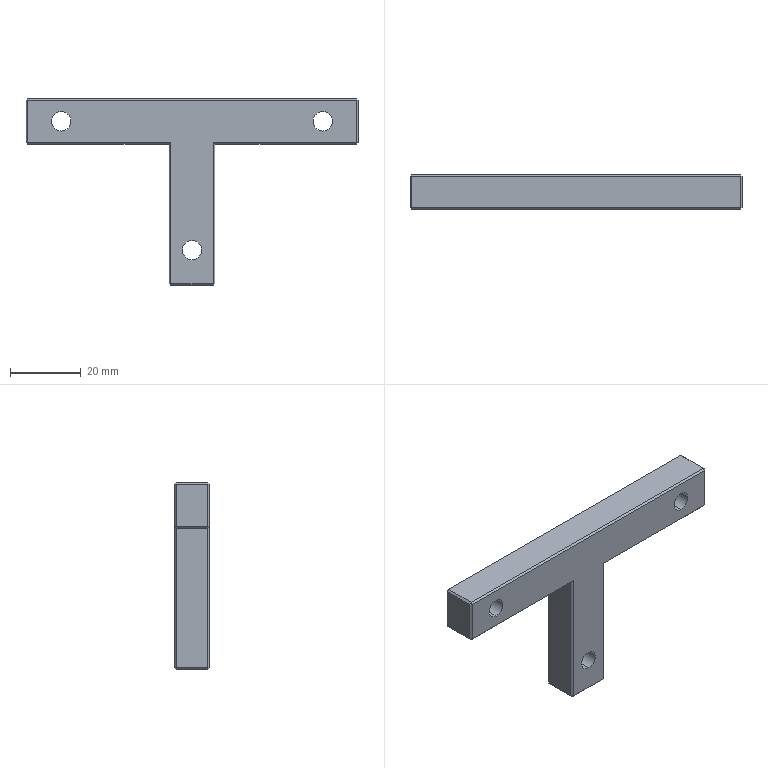Part | 1 solid | 59 faces | box 94 x 10 x 53 mm | volume 15677 mm3 | plane 47 | cylinder 12 | commonest cylinder face diameters 5.5 x6 10 x6
STEP:
#1=CARTESIAN_POINT('',(-37.,4.3,1.5));
#2=VERTEX_POINT('',#1);
#3=CARTESIAN_POINT('',(-37.,4.3,11.5));
#4=VERTEX_POINT('',#3);
#5=CARTESIAN_POINT('',(-37.,4.3,6.5));
#6=DIRECTION('',(0.,1.,0.));
#7=DIRECTION('',(0.,0.,1.));
#8=AXIS2_PLACEMENT_3D('',#5,#6,#7);
#9=CIRCLE('',#8,5.);
#10=EDGE_CURVE('',#2,#4,#9,.T.);
#11=ORIENTED_EDGE('',*,*,#10,.F.);
#12=CARTESIAN_POINT('',(-37.,10.,1.5));
#13=VERTEX_POINT('',#12);
#14=CARTESIAN_POINT('',(-37.,10.,1.5));
#15=DIRECTION('',(0.,1.,0.));
#16=VECTOR('',#15,1000.);
#17=LINE('',#14,#16);
#18=EDGE_CURVE('',#2,#13,#17,.T.);
#19=ORIENTED_EDGE('',*,*,#18,.T.);
#20=CARTESIAN_POINT('',(-37.,10.,11.5));
#21=VERTEX_POINT('',#20);
#22=CARTESIAN_POINT('',(-37.,10.,6.5));
#23=DIRECTION('',(0.,1.,0.));
#24=DIRECTION('',(0.,0.,1.));
#25=AXIS2_PLACEMENT_3D('',#22,#23,#24);
#26=CIRCLE('',#25,5.);
#27=EDGE_CURVE('',#13,#21,#26,.T.);
#28=ORIENTED_EDGE('',*,*,#27,.T.);
#29=CARTESIAN_POINT('',(-37.,10.,11.5));
#30=DIRECTION('',(0.,1.,0.));
#31=VECTOR('',#30,1000.);
#32=LINE('',#29,#31);
#33=EDGE_CURVE('',#4,#21,#32,.T.);
#34=ORIENTED_EDGE('',*,*,#33,.F.);
#35=EDGE_LOOP('',(#11,#19,#28,#34));
#36=FACE_OUTER_BOUND('',#35,.T.);
#37=CARTESIAN_POINT('',(-37.,10.,6.5));
#38=DIRECTION('',(0.,1.,0.));
#39=DIRECTION('',(0.,0.,1.));
#40=AXIS2_PLACEMENT_3D('',#37,#38,#39);
#41=CYLINDRICAL_SURFACE('',#40,5.);
#42=ADVANCED_FACE('',(#36),#41,.F.);
#43=CARTESIAN_POINT('',(-37.,0.,3.75));
#44=VERTEX_POINT('',#43);
#45=CARTESIAN_POINT('',(-37.,0.,9.25));
#46=VERTEX_POINT('',#45);
#47=CARTESIAN_POINT('',(-37.,0.,6.5));
#48=DIRECTION('',(0.,1.,0.));
#49=DIRECTION('',(0.,0.,1.));
#50=AXIS2_PLACEMENT_3D('',#47,#48,#49);
#51=CIRCLE('',#50,2.75);
#52=EDGE_CURVE('',#44,#46,#51,.T.);
#53=ORIENTED_EDGE('',*,*,#52,.F.);
#54=CARTESIAN_POINT('',(-37.,4.3,3.75));
#55=VERTEX_POINT('',#54);
#56=CARTESIAN_POINT('',(-37.,10.,3.75));
#57=DIRECTION('',(0.,1.,0.));
#58=VECTOR('',#57,1000.);
#59=LINE('',#56,#58);
#60=EDGE_CURVE('',#44,#55,#59,.T.);
#61=ORIENTED_EDGE('',*,*,#60,.T.);
#62=CARTESIAN_POINT('',(-37.,4.3,9.25));
#63=VERTEX_POINT('',#62);
#64=CARTESIAN_POINT('',(-37.,4.3,6.5));
#65=DIRECTION('',(0.,1.,0.));
#66=DIRECTION('',(0.,0.,1.));
#67=AXIS2_PLACEMENT_3D('',#64,#65,#66);
#68=CIRCLE('',#67,2.75);
#69=EDGE_CURVE('',#55,#63,#68,.T.);
#70=ORIENTED_EDGE('',*,*,#69,.T.);
#71=CARTESIAN_POINT('',(-37.,10.,9.25));
#72=DIRECTION('',(0.,1.,0.));
#73=VECTOR('',#72,1000.);
#74=LINE('',#71,#73);
#75=EDGE_CURVE('',#46,#63,#74,.T.);
#76=ORIENTED_EDGE('',*,*,#75,.F.);
#77=EDGE_LOOP('',(#53,#61,#70,#76));
#78=FACE_OUTER_BOUND('',#77,.T.);
#79=CARTESIAN_POINT('',(-37.,10.,6.5));
#80=DIRECTION('',(0.,1.,0.));
#81=DIRECTION('',(0.,0.,1.));
#82=AXIS2_PLACEMENT_3D('',#79,#80,#81);
#83=CYLINDRICAL_SURFACE('',#82,2.75);
#84=ADVANCED_FACE('',(#78),#83,.F.);
#85=CARTESIAN_POINT('',(37.,4.3,1.5));
#86=VERTEX_POINT('',#85);
#87=CARTESIAN_POINT('',(37.,4.3,11.5));
#88=VERTEX_POINT('',#87);
#89=CARTESIAN_POINT('',(37.,4.3,6.5));
#90=DIRECTION('',(0.,1.,0.));
#91=DIRECTION('',(0.,0.,1.));
#92=AXIS2_PLACEMENT_3D('',#89,#90,#91);
#93=CIRCLE('',#92,5.);
#94=EDGE_CURVE('',#86,#88,#93,.T.);
#95=ORIENTED_EDGE('',*,*,#94,.F.);
#96=CARTESIAN_POINT('',(37.,10.,1.5));
#97=VERTEX_POINT('',#96);
#98=CARTESIAN_POINT('',(37.,10.,1.5));
#99=DIRECTION('',(0.,1.,0.));
#100=VECTOR('',#99,1000.);
#101=LINE('',#98,#100);
#102=EDGE_CURVE('',#86,#97,#101,.T.);
#103=ORIENTED_EDGE('',*,*,#102,.T.);
#104=CARTESIAN_POINT('',(37.,10.,11.5));
#105=VERTEX_POINT('',#104);
#106=CARTESIAN_POINT('',(37.,10.,6.5));
#107=DIRECTION('',(0.,1.,0.));
#108=DIRECTION('',(0.,0.,1.));
#109=AXIS2_PLACEMENT_3D('',#106,#107,#108);
#110=CIRCLE('',#109,5.);
#111=EDGE_CURVE('',#97,#105,#110,.T.);
#112=ORIENTED_EDGE('',*,*,#111,.T.);
#113=CARTESIAN_POINT('',(37.,10.,11.5));
#114=DIRECTION('',(0.,1.,0.));
#115=VECTOR('',#114,1000.);
#116=LINE('',#113,#115);
#117=EDGE_CURVE('',#88,#105,#116,.T.);
#118=ORIENTED_EDGE('',*,*,#117,.F.);
#119=EDGE_LOOP('',(#95,#103,#112,#118));
#120=FACE_OUTER_BOUND('',#119,.T.);
#121=CARTESIAN_POINT('',(37.,10.,6.5));
#122=DIRECTION('',(0.,1.,0.));
#123=DIRECTION('',(0.,0.,1.));
#124=AXIS2_PLACEMENT_3D('',#121,#122,#123);
#125=CYLINDRICAL_SURFACE('',#124,5.);
#126=ADVANCED_FACE('',(#120),#125,.F.);
#127=CARTESIAN_POINT('',(37.,0.,3.75));
#128=VERTEX_POINT('',#127);
#129=CARTESIAN_POINT('',(37.,0.,9.25));
#130=VERTEX_POINT('',#129);
#131=CARTESIAN_POINT('',(37.,0.,6.5));
#132=DIRECTION('',(0.,1.,0.));
#133=DIRECTION('',(0.,0.,1.));
#134=AXIS2_PLACEMENT_3D('',#131,#132,#133);
#135=CIRCLE('',#134,2.75);
#136=EDGE_CURVE('',#128,#130,#135,.T.);
#137=ORIENTED_EDGE('',*,*,#136,.F.);
#138=CARTESIAN_POINT('',(37.,4.3,3.75));
#139=VERTEX_POINT('',#138);
#140=CARTESIAN_POINT('',(37.,10.,3.75));
#141=DIRECTION('',(0.,1.,0.));
#142=VECTOR('',#141,1000.);
#143=LINE('',#140,#142);
#144=EDGE_CURVE('',#128,#139,#143,.T.);
#145=ORIENTED_EDGE('',*,*,#144,.T.);
#146=CARTESIAN_POINT('',(37.,4.3,9.25));
#147=VERTEX_POINT('',#146);
#148=CARTESIAN_POINT('',(37.,4.3,6.5));
#149=DIRECTION('',(0.,1.,0.));
#150=DIRECTION('',(0.,0.,1.));
#151=AXIS2_PLACEMENT_3D('',#148,#149,#150);
#152=CIRCLE('',#151,2.75);
#153=EDGE_CURVE('',#139,#147,#152,.T.);
#154=ORIENTED_EDGE('',*,*,#153,.T.);
#155=CARTESIAN_POINT('',(37.,10.,9.25));
#156=DIRECTION('',(0.,1.,0.));
#157=VECTOR('',#156,1000.);
#158=LINE('',#155,#157);
#159=EDGE_CURVE('',#130,#147,#158,.T.);
#160=ORIENTED_EDGE('',*,*,#159,.F.);
#161=EDGE_LOOP('',(#137,#145,#154,#160));
#162=FACE_OUTER_BOUND('',#161,.T.);
#163=CARTESIAN_POINT('',(37.,10.,6.5));
#164=DIRECTION('',(0.,1.,0.));
#165=DIRECTION('',(0.,0.,1.));
#166=AXIS2_PLACEMENT_3D('',#163,#164,#165);
#167=CYLINDRICAL_SURFACE('',#166,2.75);
#168=ADVANCED_FACE('',(#162),#167,.F.);
#169=CARTESIAN_POINT('',(0.,4.3,-35.));
#170=VERTEX_POINT('',#169);
#171=CARTESIAN_POINT('',(0.,4.3,-25.));
#172=VERTEX_POINT('',#171);
#173=CARTESIAN_POINT('',(0.,4.3,-30.));
#174=DIRECTION('',(0.,1.,0.));
#175=DIRECTION('',(0.,0.,1.));
#176=AXIS2_PLACEMENT_3D('',#173,#174,#175);
#177=CIRCLE('',#176,5.);
#178=EDGE_CURVE('',#170,#172,#177,.T.);
#179=ORIENTED_EDGE('',*,*,#178,.F.);
#180=CARTESIAN_POINT('',(0.,10.,-35.));
#181=VERTEX_POINT('',#180);
#182=CARTESIAN_POINT('',(0.,10.,-35.));
#183=DIRECTION('',(0.,1.,0.));
#184=VECTOR('',#183,1000.);
#185=LINE('',#182,#184);
#186=EDGE_CURVE('',#170,#181,#185,.T.);
#187=ORIENTED_EDGE('',*,*,#186,.T.);
#188=CARTESIAN_POINT('',(0.,10.,-25.));
#189=VERTEX_POINT('',#188);
#190=CARTESIAN_POINT('',(0.,10.,-30.));
#191=DIRECTION('',(0.,1.,0.));
#192=DIRECTION('',(0.,0.,1.));
#193=AXIS2_PLACEMENT_3D('',#190,#191,#192);
#194=CIRCLE('',#193,5.);
#195=EDGE_CURVE('',#181,#189,#194,.T.);
#196=ORIENTED_EDGE('',*,*,#195,.T.);
#197=CARTESIAN_POINT('',(0.,10.,-25.));
#198=DIRECTION('',(0.,1.,0.));
#199=VECTOR('',#198,1000.);
#200=LINE('',#197,#199);
#201=EDGE_CURVE('',#172,#189,#200,.T.);
#202=ORIENTED_EDGE('',*,*,#201,.F.);
#203=EDGE_LOOP('',(#179,#187,#196,#202));
#204=FACE_OUTER_BOUND('',#203,.T.);
#205=CARTESIAN_POINT('',(0.,10.,-30.));
#206=DIRECTION('',(0.,1.,0.));
#207=DIRECTION('',(0.,0.,1.));
#208=AXIS2_PLACEMENT_3D('',#205,#206,#207);
#209=CYLINDRICAL_SURFACE('',#208,5.);
#210=ADVANCED_FACE('',(#204),#209,.F.);
#211=CARTESIAN_POINT('',(0.,0.,-32.75));
#212=VERTEX_POINT('',#211);
#213=CARTESIAN_POINT('',(0.,0.,-27.25));
#214=VERTEX_POINT('',#213);
#215=CARTESIAN_POINT('',(0.,0.,-30.));
#216=DIRECTION('',(0.,1.,0.));
#217=DIRECTION('',(0.,0.,1.));
#218=AXIS2_PLACEMENT_3D('',#215,#216,#217);
#219=CIRCLE('',#218,2.75);
#220=EDGE_CURVE('',#212,#214,#219,.T.);
#221=ORIENTED_EDGE('',*,*,#220,.F.);
#222=CARTESIAN_POINT('',(0.,4.3,-32.75));
#223=VERTEX_POINT('',#222);
#224=CARTESIAN_POINT('',(0.,10.,-32.75));
#225=DIRECTION('',(0.,1.,0.));
#226=VECTOR('',#225,1000.);
#227=LINE('',#224,#226);
#228=EDGE_CURVE('',#212,#223,#227,.T.);
#229=ORIENTED_EDGE('',*,*,#228,.T.);
#230=CARTESIAN_POINT('',(0.,4.3,-27.25));
#231=VERTEX_POINT('',#230);
#232=CARTESIAN_POINT('',(0.,4.3,-30.));
#233=DIRECTION('',(0.,1.,0.));
#234=DIRECTION('',(0.,0.,1.));
#235=AXIS2_PLACEMENT_3D('',#232,#233,#234);
#236=CIRCLE('',#235,2.75);
#237=EDGE_CURVE('',#223,#231,#236,.T.);
#238=ORIENTED_EDGE('',*,*,#237,.T.);
#239=CARTESIAN_POINT('',(0.,10.,-27.25));
#240=DIRECTION('',(0.,1.,0.));
#241=VECTOR('',#240,1000.);
#242=LINE('',#239,#241);
#243=EDGE_CURVE('',#214,#231,#242,.T.);
#244=ORIENTED_EDGE('',*,*,#243,.F.);
#245=EDGE_LOOP('',(#221,#229,#238,#244));
#246=FACE_OUTER_BOUND('',#245,.T.);
#247=CARTESIAN_POINT('',(0.,10.,-30.));
#248=DIRECTION('',(0.,1.,0.));
#249=DIRECTION('',(0.,0.,1.));
#250=AXIS2_PLACEMENT_3D('',#247,#248,#249);
#251=CYLINDRICAL_SURFACE('',#250,2.75);
#252=ADVANCED_FACE('',(#246),#251,.F.);
#253=CARTESIAN_POINT('',(-47.,0.54,0.54));
#254=VERTEX_POINT('',#253);
#255=CARTESIAN_POINT('',(-47.,0.54,12.46));
#256=VERTEX_POINT('',#255);
#257=CARTESIAN_POINT('',(-47.,0.54,13.));
#258=DIRECTION('',(0.,0.,1.));
#259=VECTOR('',#258,1000.);
#260=LINE('',#257,#259);
#261=EDGE_CURVE('',#254,#256,#260,.T.);
#262=ORIENTED_EDGE('',*,*,#261,.T.);
#263=CARTESIAN_POINT('',(-47.,9.46,12.46));
#264=VERTEX_POINT('',#263);
#265=CARTESIAN_POINT('',(-47.,10.,12.46));
#266=DIRECTION('',(0.,1.,0.));
#267=VECTOR('',#266,1000.);
#268=LINE('',#265,#267);
#269=EDGE_CURVE('',#256,#264,#268,.T.);
#270=ORIENTED_EDGE('',*,*,#269,.T.);
#271=CARTESIAN_POINT('',(-47.,9.46,0.54));
#272=VERTEX_POINT('',#271);
#273=CARTESIAN_POINT('',(-47.,9.46,13.));
#274=DIRECTION('',(0.,0.,-1.));
#275=VECTOR('',#274,1000.);
#276=LINE('',#273,#275);
#277=EDGE_CURVE('',#264,#272,#276,.T.);
#278=ORIENTED_EDGE('',*,*,#277,.T.);
#279=CARTESIAN_POINT('',(-47.,10.,0.54));
#280=DIRECTION('',(0.,-1.,0.));
#281=VECTOR('',#280,1000.);
#282=LINE('',#279,#281);
#283=EDGE_CURVE('',#272,#254,#282,.T.);
#284=ORIENTED_EDGE('',*,*,#283,.T.);
#285=EDGE_LOOP('',(#262,#270,#278,#284));
#286=FACE_OUTER_BOUND('',#285,.T.);
#287=CARTESIAN_POINT('',(-47.,10.,13.));
#288=DIRECTION('',(1.,0.,0.));
#289=DIRECTION('',(0.,0.,-1.));
#290=AXIS2_PLACEMENT_3D('',#287,#288,#289);
#291=PLANE('',#290);
#292=ADVANCED_FACE('',(#286),#291,.F.);
#293=CARTESIAN_POINT('',(46.46,9.46,13.));
#294=VERTEX_POINT('',#293);
#295=CARTESIAN_POINT('',(-46.46,9.46,13.));
#296=VERTEX_POINT('',#295);
#297=CARTESIAN_POINT('',(47.,9.46,13.));
#298=DIRECTION('',(-1.,0.,0.));
#299=VECTOR('',#298,1000.);
#300=LINE('',#297,#299);
#301=EDGE_CURVE('',#294,#296,#300,.T.);
#302=ORIENTED_EDGE('',*,*,#301,.T.);
#303=CARTESIAN_POINT('',(-46.46,0.54,13.));
#304=VERTEX_POINT('',#303);
#305=CARTESIAN_POINT('',(-46.46,10.,13.));
#306=DIRECTION('',(0.,-1.,0.));
#307=VECTOR('',#306,1000.);
#308=LINE('',#305,#307);
#309=EDGE_CURVE('',#296,#304,#308,.T.);
#310=ORIENTED_EDGE('',*,*,#309,.T.);
#311=CARTESIAN_POINT('',(46.46,0.54,13.));
#312=VERTEX_POINT('',#311);
#313=CARTESIAN_POINT('',(47.,0.54,13.));
#314=DIRECTION('',(1.,0.,0.));
#315=VECTOR('',#314,1000.);
#316=LINE('',#313,#315);
#317=EDGE_CURVE('',#304,#312,#316,.T.);
#318=ORIENTED_EDGE('',*,*,#317,.T.);
#319=CARTESIAN_POINT('',(46.46,10.,13.));
#320=DIRECTION('',(0.,1.,0.));
#321=VECTOR('',#320,1000.);
#322=LINE('',#319,#321);
#323=EDGE_CURVE('',#312,#294,#322,.T.);
#324=ORIENTED_EDGE('',*,*,#323,.T.);
#325=EDGE_LOOP('',(#302,#310,#318,#324));
#326=FACE_OUTER_BOUND('',#325,.T.);
#327=CARTESIAN_POINT('',(47.,10.,13.));
#328=DIRECTION('',(0.,0.,-1.));
#329=DIRECTION('',(-1.,0.,0.));
#330=AXIS2_PLACEMENT_3D('',#327,#328,#329);
#331=PLANE('',#330);
#332=ADVANCED_FACE('',(#326),#331,.F.);
#333=CARTESIAN_POINT('',(47.,9.46,0.54));
#334=VERTEX_POINT('',#333);
#335=CARTESIAN_POINT('',(47.,9.46,12.46));
#336=VERTEX_POINT('',#335);
#337=CARTESIAN_POINT('',(47.,9.46,0.));
#338=DIRECTION('',(0.,0.,1.));
#339=VECTOR('',#338,1000.);
#340=LINE('',#337,#339);
#341=EDGE_CURVE('',#334,#336,#340,.T.);
#342=ORIENTED_EDGE('',*,*,#341,.T.);
#343=CARTESIAN_POINT('',(47.,0.54,12.46));
#344=VERTEX_POINT('',#343);
#345=CARTESIAN_POINT('',(47.,10.,12.46));
#346=DIRECTION('',(0.,-1.,0.));
#347=VECTOR('',#346,1000.);
#348=LINE('',#345,#347);
#349=EDGE_CURVE('',#336,#344,#348,.T.);
#350=ORIENTED_EDGE('',*,*,#349,.T.);
#351=CARTESIAN_POINT('',(47.,0.54,0.54));
#352=VERTEX_POINT('',#351);
#353=CARTESIAN_POINT('',(47.,0.54,0.));
#354=DIRECTION('',(0.,0.,-1.));
#355=VECTOR('',#354,1000.);
#356=LINE('',#353,#355);
#357=EDGE_CURVE('',#344,#352,#356,.T.);
#358=ORIENTED_EDGE('',*,*,#357,.T.);
#359=CARTESIAN_POINT('',(47.,10.,0.54));
#360=DIRECTION('',(0.,1.,0.));
#361=VECTOR('',#360,1000.);
#362=LINE('',#359,#361);
#363=EDGE_CURVE('',#352,#334,#362,.T.);
#364=ORIENTED_EDGE('',*,*,#363,.T.);
#365=EDGE_LOOP('',(#342,#350,#358,#364));
#366=FACE_OUTER_BOUND('',#365,.T.);
#367=CARTESIAN_POINT('',(47.,10.,0.));
#368=DIRECTION('',(-1.,0.,0.));
#369=DIRECTION('',(0.,0.,1.));
#370=AXIS2_PLACEMENT_3D('',#367,#368,#369);
#371=PLANE('',#370);
#372=ADVANCED_FACE('',(#366),#371,.F.);
#373=CARTESIAN_POINT('',(46.46,9.46,0.));
#374=VERTEX_POINT('',#373);
#375=CARTESIAN_POINT('',(46.46,0.54,0.));
#376=VERTEX_POINT('',#375);
#377=CARTESIAN_POINT('',(46.46,10.,0.));
#378=DIRECTION('',(0.,-1.,0.));
#379=VECTOR('',#378,1000.);
#380=LINE('',#377,#379);
#381=EDGE_CURVE('',#374,#376,#380,.T.);
#382=ORIENTED_EDGE('',*,*,#381,.T.);
#383=CARTESIAN_POINT('',(6.5,0.54,0.));
#384=VERTEX_POINT('',#383);
#385=CARTESIAN_POINT('',(6.5,0.54,0.));
#386=DIRECTION('',(-1.,0.,0.));
#387=VECTOR('',#386,1000.);
#388=LINE('',#385,#387);
#389=EDGE_CURVE('',#376,#384,#388,.T.);
#390=ORIENTED_EDGE('',*,*,#389,.T.);
#391=CARTESIAN_POINT('',(6.5,9.46,0.));
#392=VERTEX_POINT('',#391);
#393=CARTESIAN_POINT('',(6.5,10.,0.));
#394=DIRECTION('',(0.,-1.,0.));
#395=VECTOR('',#394,1000.);
#396=LINE('',#393,#395);
#397=EDGE_CURVE('',#392,#384,#396,.T.);
#398=ORIENTED_EDGE('',*,*,#397,.F.);
#399=CARTESIAN_POINT('',(6.5,9.46,0.));
#400=DIRECTION('',(1.,0.,0.));
#401=VECTOR('',#400,1000.);
#402=LINE('',#399,#401);
#403=EDGE_CURVE('',#392,#374,#402,.T.);
#404=ORIENTED_EDGE('',*,*,#403,.T.);
#405=EDGE_LOOP('',(#382,#390,#398,#404));
#406=FACE_OUTER_BOUND('',#405,.T.);
#407=CARTESIAN_POINT('',(6.5,10.,0.));
#408=DIRECTION('',(0.,0.,1.));
#409=DIRECTION('',(1.,0.,0.));
#410=AXIS2_PLACEMENT_3D('',#407,#408,#409);
#411=PLANE('',#410);
#412=ADVANCED_FACE('',(#406),#411,.F.);
#413=ORIENTED_EDGE('',*,*,#397,.T.);
#414=CARTESIAN_POINT('',(6.5,0.54,-39.46));
#415=VERTEX_POINT('',#414);
#416=CARTESIAN_POINT('',(6.5,0.54,-40.));
#417=DIRECTION('',(0.,0.,-1.));
#418=VECTOR('',#417,1000.);
#419=LINE('',#416,#418);
#420=EDGE_CURVE('',#384,#415,#419,.T.);
#421=ORIENTED_EDGE('',*,*,#420,.T.);
#422=CARTESIAN_POINT('',(6.5,9.46,-39.46));
#423=VERTEX_POINT('',#422);
#424=CARTESIAN_POINT('',(6.5,10.,-39.46));
#425=DIRECTION('',(0.,1.,0.));
#426=VECTOR('',#425,1000.);
#427=LINE('',#424,#426);
#428=EDGE_CURVE('',#415,#423,#427,.T.);
#429=ORIENTED_EDGE('',*,*,#428,.T.);
#430=CARTESIAN_POINT('',(6.5,9.46,-40.));
#431=DIRECTION('',(0.,0.,1.));
#432=VECTOR('',#431,1000.);
#433=LINE('',#430,#432);
#434=EDGE_CURVE('',#423,#392,#433,.T.);
#435=ORIENTED_EDGE('',*,*,#434,.T.);
#436=EDGE_LOOP('',(#413,#421,#429,#435));
#437=FACE_OUTER_BOUND('',#436,.T.);
#438=CARTESIAN_POINT('',(6.5,10.,-40.));
#439=DIRECTION('',(-1.,0.,0.));
#440=DIRECTION('',(0.,0.,1.));
#441=AXIS2_PLACEMENT_3D('',#438,#439,#440);
#442=PLANE('',#441);
#443=ADVANCED_FACE('',(#437),#442,.F.);
#444=CARTESIAN_POINT('',(5.96,9.46,-40.));
#445=VERTEX_POINT('',#444);
#446=CARTESIAN_POINT('',(5.96,0.54,-40.));
#447=VERTEX_POINT('',#446);
#448=CARTESIAN_POINT('',(5.96,10.,-40.));
#449=DIRECTION('',(0.,-1.,0.));
#450=VECTOR('',#449,1000.);
#451=LINE('',#448,#450);
#452=EDGE_CURVE('',#445,#447,#451,.T.);
#453=ORIENTED_EDGE('',*,*,#452,.T.);
#454=CARTESIAN_POINT('',(-5.96,0.54,-40.));
#455=VERTEX_POINT('',#454);
#456=CARTESIAN_POINT('',(-6.5,0.54,-40.));
#457=DIRECTION('',(-1.,0.,0.));
#458=VECTOR('',#457,1000.);
#459=LINE('',#456,#458);
#460=EDGE_CURVE('',#447,#455,#459,.T.);
#461=ORIENTED_EDGE('',*,*,#460,.T.);
#462=CARTESIAN_POINT('',(-5.96,9.46,-40.));
#463=VERTEX_POINT('',#462);
#464=CARTESIAN_POINT('',(-5.96,10.,-40.));
#465=DIRECTION('',(0.,1.,0.));
#466=VECTOR('',#465,1000.);
#467=LINE('',#464,#466);
#468=EDGE_CURVE('',#455,#463,#467,.T.);
#469=ORIENTED_EDGE('',*,*,#468,.T.);
#470=CARTESIAN_POINT('',(-6.5,9.46,-40.));
#471=DIRECTION('',(1.,0.,0.));
#472=VECTOR('',#471,1000.);
#473=LINE('',#470,#472);
#474=EDGE_CURVE('',#463,#445,#473,.T.);
#475=ORIENTED_EDGE('',*,*,#474,.T.);
#476=EDGE_LOOP('',(#453,#461,#469,#475));
#477=FACE_OUTER_BOUND('',#476,.T.);
#478=CARTESIAN_POINT('',(-6.5,10.,-40.));
#479=DIRECTION('',(0.,0.,1.));
#480=DIRECTION('',(1.,0.,0.));
#481=AXIS2_PLACEMENT_3D('',#478,#479,#480);
#482=PLANE('',#481);
#483=ADVANCED_FACE('',(#477),#482,.F.);
#484=CARTESIAN_POINT('',(-6.5,9.46,-39.46));
#485=VERTEX_POINT('',#484);
#486=CARTESIAN_POINT('',(-6.5,0.54,-39.46));
#487=VERTEX_POINT('',#486);
#488=CARTESIAN_POINT('',(-6.5,10.,-39.46));
#489=DIRECTION('',(0.,-1.,0.));
#490=VECTOR('',#489,1000.);
#491=LINE('',#488,#490);
#492=EDGE_CURVE('',#485,#487,#491,.T.);
#493=ORIENTED_EDGE('',*,*,#492,.T.);
#494=CARTESIAN_POINT('',(-6.5,0.54,0.));
#495=VERTEX_POINT('',#494);
#496=CARTESIAN_POINT('',(-6.5,0.54,0.));
#497=DIRECTION('',(0.,0.,1.));
#498=VECTOR('',#497,1000.);
#499=LINE('',#496,#498);
#500=EDGE_CURVE('',#487,#495,#499,.T.);
#501=ORIENTED_EDGE('',*,*,#500,.T.);
#502=CARTESIAN_POINT('',(-6.5,9.46,0.));
#503=VERTEX_POINT('',#502);
#504=CARTESIAN_POINT('',(-6.5,10.,0.));
#505=DIRECTION('',(0.,-1.,0.));
#506=VECTOR('',#505,1000.);
#507=LINE('',#504,#506);
#508=EDGE_CURVE('',#503,#495,#507,.T.);
#509=ORIENTED_EDGE('',*,*,#508,.F.);
#510=CARTESIAN_POINT('',(-6.5,9.46,0.));
#511=DIRECTION('',(0.,0.,-1.));
#512=VECTOR('',#511,1000.);
#513=LINE('',#510,#512);
#514=EDGE_CURVE('',#503,#485,#513,.T.);
#515=ORIENTED_EDGE('',*,*,#514,.T.);
#516=EDGE_LOOP('',(#493,#501,#509,#515));
#517=FACE_OUTER_BOUND('',#516,.T.);
#518=CARTESIAN_POINT('',(-6.5,10.,0.));
#519=DIRECTION('',(1.,0.,0.));
#520=DIRECTION('',(0.,0.,-1.));
#521=AXIS2_PLACEMENT_3D('',#518,#519,#520);
#522=PLANE('',#521);
#523=ADVANCED_FACE('',(#517),#522,.F.);
#524=ORIENTED_EDGE('',*,*,#508,.T.);
#525=CARTESIAN_POINT('',(-46.46,0.54,0.));
#526=VERTEX_POINT('',#525);
#527=CARTESIAN_POINT('',(-47.,0.54,0.));
#528=DIRECTION('',(-1.,0.,0.));
#529=VECTOR('',#528,1000.);
#530=LINE('',#527,#529);
#531=EDGE_CURVE('',#495,#526,#530,.T.);
#532=ORIENTED_EDGE('',*,*,#531,.T.);
#533=CARTESIAN_POINT('',(-46.46,9.46,0.));
#534=VERTEX_POINT('',#533);
#535=CARTESIAN_POINT('',(-46.46,10.,0.));
#536=DIRECTION('',(0.,1.,0.));
#537=VECTOR('',#536,1000.);
#538=LINE('',#535,#537);
#539=EDGE_CURVE('',#526,#534,#538,.T.);
#540=ORIENTED_EDGE('',*,*,#539,.T.);
#541=CARTESIAN_POINT('',(-47.,9.46,0.));
#542=DIRECTION('',(1.,0.,0.));
#543=VECTOR('',#542,1000.);
#544=LINE('',#541,#543);
#545=EDGE_CURVE('',#534,#503,#544,.T.);
#546=ORIENTED_EDGE('',*,*,#545,.T.);
#547=EDGE_LOOP('',(#524,#532,#540,#546));
#548=FACE_OUTER_BOUND('',#547,.T.);
#549=CARTESIAN_POINT('',(-47.,10.,0.));
#550=DIRECTION('',(0.,0.,1.));
#551=DIRECTION('',(1.,0.,0.));
#552=AXIS2_PLACEMENT_3D('',#549,#550,#551);
#553=PLANE('',#552);
#554=ADVANCED_FACE('',(#548),#553,.F.);
#555=CARTESIAN_POINT('',(-37.,10.,6.5));
#556=DIRECTION('',(0.,1.,0.));
#557=DIRECTION('',(0.,0.,1.));
#558=AXIS2_PLACEMENT_3D('',#555,#556,#557);
#559=CIRCLE('',#558,5.);
#560=EDGE_CURVE('',#21,#13,#559,.T.);
#561=ORIENTED_EDGE('',*,*,#560,.F.);
#562=ORIENTED_EDGE('',*,*,#27,.F.);
#563=EDGE_LOOP('',(#561,#562));
#564=FACE_BOUND('',#563,.T.);
#565=CARTESIAN_POINT('',(37.,10.,6.5));
#566=DIRECTION('',(0.,1.,0.));
#567=DIRECTION('',(0.,0.,1.));
#568=AXIS2_PLACEMENT_3D('',#565,#566,#567);
#569=CIRCLE('',#568,5.);
#570=EDGE_CURVE('',#105,#97,#569,.T.);
#571=ORIENTED_EDGE('',*,*,#570,.F.);
#572=ORIENTED_EDGE('',*,*,#111,.F.);
#573=EDGE_LOOP('',(#571,#572));
#574=FACE_BOUND('',#573,.T.);
#575=CARTESIAN_POINT('',(0.,10.,-30.));
#576=DIRECTION('',(0.,1.,0.));
#577=DIRECTION('',(0.,0.,1.));
#578=AXIS2_PLACEMENT_3D('',#575,#576,#577);
#579=CIRCLE('',#578,5.);
#580=EDGE_CURVE('',#189,#181,#579,.T.);
#581=ORIENTED_EDGE('',*,*,#580,.F.);
#582=ORIENTED_EDGE('',*,*,#195,.F.);
#583=EDGE_LOOP('',(#581,#582));
#584=FACE_BOUND('',#583,.T.);
#585=CARTESIAN_POINT('',(-46.46,10.,0.54));
#586=VERTEX_POINT('',#585);
#587=CARTESIAN_POINT('',(-46.46,10.,12.46));
#588=VERTEX_POINT('',#587);
#589=CARTESIAN_POINT('',(-46.46,10.,0.));
#590=DIRECTION('',(0.,0.,1.));
#591=VECTOR('',#590,1000.);
#592=LINE('',#589,#591);
#593=EDGE_CURVE('',#586,#588,#592,.T.);
#594=ORIENTED_EDGE('',*,*,#593,.T.);
#595=CARTESIAN_POINT('',(46.46,10.,12.46));
#596=VERTEX_POINT('',#595);
#597=CARTESIAN_POINT('',(0.,10.,12.46));
#598=DIRECTION('',(1.,0.,0.));
#599=VECTOR('',#598,1000.);
#600=LINE('',#597,#599);
#601=EDGE_CURVE('',#588,#596,#600,.T.);
#602=ORIENTED_EDGE('',*,*,#601,.T.);
#603=CARTESIAN_POINT('',(46.46,10.,0.54));
#604=VERTEX_POINT('',#603);
#605=CARTESIAN_POINT('',(46.46,10.,0.));
#606=DIRECTION('',(0.,0.,-1.));
#607=VECTOR('',#606,1000.);
#608=LINE('',#605,#607);
#609=EDGE_CURVE('',#596,#604,#608,.T.);
#610=ORIENTED_EDGE('',*,*,#609,.T.);
#611=CARTESIAN_POINT('',(5.96,10.,0.54));
#612=VERTEX_POINT('',#611);
#613=CARTESIAN_POINT('',(0.,10.,0.54));
#614=DIRECTION('',(-1.,0.,0.));
#615=VECTOR('',#614,1000.);
#616=LINE('',#613,#615);
#617=EDGE_CURVE('',#604,#612,#616,.T.);
#618=ORIENTED_EDGE('',*,*,#617,.T.);
#619=CARTESIAN_POINT('',(5.96,10.,-39.46));
#620=VERTEX_POINT('',#619);
#621=CARTESIAN_POINT('',(5.96,10.,0.));
#622=DIRECTION('',(0.,0.,-1.));
#623=VECTOR('',#622,1000.);
#624=LINE('',#621,#623);
#625=EDGE_CURVE('',#612,#620,#624,.T.);
#626=ORIENTED_EDGE('',*,*,#625,.T.);
#627=CARTESIAN_POINT('',(-5.96,10.,-39.46));
#628=VERTEX_POINT('',#627);
#629=CARTESIAN_POINT('',(0.,10.,-39.46));
#630=DIRECTION('',(-1.,0.,0.));
#631=VECTOR('',#630,1000.);
#632=LINE('',#629,#631);
#633=EDGE_CURVE('',#620,#628,#632,.T.);
#634=ORIENTED_EDGE('',*,*,#633,.T.);
#635=CARTESIAN_POINT('',(-5.96,10.,0.54));
#636=VERTEX_POINT('',#635);
#637=CARTESIAN_POINT('',(-5.96,10.,0.));
#638=DIRECTION('',(0.,0.,1.));
#639=VECTOR('',#638,1000.);
#640=LINE('',#637,#639);
#641=EDGE_CURVE('',#628,#636,#640,.T.);
#642=ORIENTED_EDGE('',*,*,#641,.T.);
#643=CARTESIAN_POINT('',(0.,10.,0.54));
#644=DIRECTION('',(-1.,0.,0.));
#645=VECTOR('',#644,1000.);
#646=LINE('',#643,#645);
#647=EDGE_CURVE('',#636,#586,#646,.T.);
#648=ORIENTED_EDGE('',*,*,#647,.T.);
#649=EDGE_LOOP('',(#594,#602,#610,#618,#626,#634,#642,#648));
#650=FACE_OUTER_BOUND('',#649,.T.);
#651=CARTESIAN_POINT('',(0.,10.,0.));
#652=DIRECTION('',(0.,-1.,0.));
#653=DIRECTION('',(0.,0.,-1.));
#654=AXIS2_PLACEMENT_3D('',#651,#652,#653);
#655=PLANE('',#654);
#656=ADVANCED_FACE('',(#564,#574,#584,#650),#655,.F.);
#657=CARTESIAN_POINT('',(-37.,0.,6.5));
#658=DIRECTION('',(0.,1.,0.));
#659=DIRECTION('',(0.,0.,1.));
#660=AXIS2_PLACEMENT_3D('',#657,#658,#659);
#661=CIRCLE('',#660,2.75);
#662=EDGE_CURVE('',#46,#44,#661,.T.);
#663=ORIENTED_EDGE('',*,*,#662,.T.);
#664=ORIENTED_EDGE('',*,*,#52,.T.);
#665=EDGE_LOOP('',(#663,#664));
#666=FACE_BOUND('',#665,.T.);
#667=CARTESIAN_POINT('',(37.,0.,6.5));
#668=DIRECTION('',(0.,1.,0.));
#669=DIRECTION('',(0.,0.,1.));
#670=AXIS2_PLACEMENT_3D('',#667,#668,#669);
#671=CIRCLE('',#670,2.75);
#672=EDGE_CURVE('',#130,#128,#671,.T.);
#673=ORIENTED_EDGE('',*,*,#672,.T.);
#674=ORIENTED_EDGE('',*,*,#136,.T.);
#675=EDGE_LOOP('',(#673,#674));
#676=FACE_BOUND('',#675,.T.);
#677=CARTESIAN_POINT('',(0.,0.,-30.));
#678=DIRECTION('',(0.,1.,0.));
#679=DIRECTION('',(0.,0.,1.));
#680=AXIS2_PLACEMENT_3D('',#677,#678,#679);
#681=CIRCLE('',#680,2.75);
#682=EDGE_CURVE('',#214,#212,#681,.T.);
#683=ORIENTED_EDGE('',*,*,#682,.T.);
#684=ORIENTED_EDGE('',*,*,#220,.T.);
#685=EDGE_LOOP('',(#683,#684));
#686=FACE_BOUND('',#685,.T.);
#687=CARTESIAN_POINT('',(5.96,0.,-39.46));
#688=VERTEX_POINT('',#687);
#689=CARTESIAN_POINT('',(5.96,0.,0.54));
#690=VERTEX_POINT('',#689);
#691=CARTESIAN_POINT('',(5.96,0.,0.));
#692=DIRECTION('',(0.,0.,1.));
#693=VECTOR('',#692,1000.);
#694=LINE('',#691,#693);
#695=EDGE_CURVE('',#688,#690,#694,.T.);
#696=ORIENTED_EDGE('',*,*,#695,.T.);
#697=CARTESIAN_POINT('',(46.46,0.,0.54));
#698=VERTEX_POINT('',#697);
#699=CARTESIAN_POINT('',(47.,0.,0.54));
#700=DIRECTION('',(1.,0.,0.));
#701=VECTOR('',#700,1000.);
#702=LINE('',#699,#701);
#703=EDGE_CURVE('',#690,#698,#702,.T.);
#704=ORIENTED_EDGE('',*,*,#703,.T.);
#705=CARTESIAN_POINT('',(46.46,0.,12.46));
#706=VERTEX_POINT('',#705);
#707=CARTESIAN_POINT('',(46.46,0.,13.));
#708=DIRECTION('',(0.,0.,1.));
#709=VECTOR('',#708,1000.);
#710=LINE('',#707,#709);
#711=EDGE_CURVE('',#698,#706,#710,.T.);
#712=ORIENTED_EDGE('',*,*,#711,.T.);
#713=CARTESIAN_POINT('',(-46.46,0.,12.46));
#714=VERTEX_POINT('',#713);
#715=CARTESIAN_POINT('',(-47.,0.,12.46));
#716=DIRECTION('',(-1.,0.,0.));
#717=VECTOR('',#716,1000.);
#718=LINE('',#715,#717);
#719=EDGE_CURVE('',#706,#714,#718,.T.);
#720=ORIENTED_EDGE('',*,*,#719,.T.);
#721=CARTESIAN_POINT('',(-46.46,0.,0.54));
#722=VERTEX_POINT('',#721);
#723=CARTESIAN_POINT('',(-46.46,0.,0.));
#724=DIRECTION('',(0.,0.,-1.));
#725=VECTOR('',#724,1000.);
#726=LINE('',#723,#725);
#727=EDGE_CURVE('',#714,#722,#726,.T.);
#728=ORIENTED_EDGE('',*,*,#727,.T.);
#729=CARTESIAN_POINT('',(-5.96,0.,0.54));
#730=VERTEX_POINT('',#729);
#731=CARTESIAN_POINT('',(-6.5,0.,0.54));
#732=DIRECTION('',(1.,0.,0.));
#733=VECTOR('',#732,1000.);
#734=LINE('',#731,#733);
#735=EDGE_CURVE('',#722,#730,#734,.T.);
#736=ORIENTED_EDGE('',*,*,#735,.T.);
#737=CARTESIAN_POINT('',(-5.96,0.,-39.46));
#738=VERTEX_POINT('',#737);
#739=CARTESIAN_POINT('',(-5.96,0.,-40.));
#740=DIRECTION('',(0.,0.,-1.));
#741=VECTOR('',#740,1000.);
#742=LINE('',#739,#741);
#743=EDGE_CURVE('',#730,#738,#742,.T.);
#744=ORIENTED_EDGE('',*,*,#743,.T.);
#745=CARTESIAN_POINT('',(6.5,0.,-39.46));
#746=DIRECTION('',(1.,0.,0.));
#747=VECTOR('',#746,1000.);
#748=LINE('',#745,#747);
#749=EDGE_CURVE('',#738,#688,#748,.T.);
#750=ORIENTED_EDGE('',*,*,#749,.T.);
#751=EDGE_LOOP('',(#696,#704,#712,#720,#728,#736,#744,#750));
#752=FACE_OUTER_BOUND('',#751,.T.);
#753=CARTESIAN_POINT('',(0.,0.,0.));
#754=DIRECTION('',(0.,-1.,0.));
#755=DIRECTION('',(0.,0.,-1.));
#756=AXIS2_PLACEMENT_3D('',#753,#754,#755);
#757=PLANE('',#756);
#758=ADVANCED_FACE('',(#666,#676,#686,#752),#757,.T.);
#759=CARTESIAN_POINT('',(6.5,9.46,-39.46));
#760=DIRECTION('',(-0.7071,0.,-0.7071));
#761=VECTOR('',#760,1000.);
#762=LINE('',#759,#761);
#763=EDGE_CURVE('',#423,#445,#762,.T.);
#764=ORIENTED_EDGE('',*,*,#763,.F.);
#765=ORIENTED_EDGE('',*,*,#428,.F.);
#766=CARTESIAN_POINT('',(5.96,0.54,-40.));
#767=DIRECTION('',(0.7071,0.,0.7071));
#768=VECTOR('',#767,1000.);
#769=LINE('',#766,#768);
#770=EDGE_CURVE('',#447,#415,#769,.T.);
#771=ORIENTED_EDGE('',*,*,#770,.F.);
#772=ORIENTED_EDGE('',*,*,#452,.F.);
#773=EDGE_LOOP('',(#764,#765,#771,#772));
#774=FACE_OUTER_BOUND('',#773,.T.);
#775=CARTESIAN_POINT('',(5.96,10.,-40.));
#776=DIRECTION('',(-0.7071,0.,0.7071));
#777=DIRECTION('',(0.,-1.,0.));
#778=AXIS2_PLACEMENT_3D('',#775,#776,#777);
#779=PLANE('',#778);
#780=ADVANCED_FACE('',(#774),#779,.F.);
#781=CARTESIAN_POINT('',(6.5,9.46,-39.46));
#782=DIRECTION('',(-0.7071,0.7071,0.));
#783=VECTOR('',#782,1000.);
#784=LINE('',#781,#783);
#785=EDGE_CURVE('',#423,#620,#784,.T.);
#786=ORIENTED_EDGE('',*,*,#785,.F.);
#787=ORIENTED_EDGE('',*,*,#763,.T.);
#788=CARTESIAN_POINT('',(5.96,9.73,-39.73));
#789=DIRECTION('',(0.,-0.7071,-0.7071));
#790=VECTOR('',#789,1000.);
#791=LINE('',#788,#790);
#792=EDGE_CURVE('',#620,#445,#791,.T.);
#793=ORIENTED_EDGE('',*,*,#792,.F.);
#794=EDGE_LOOP('',(#786,#787,#793));
#795=FACE_OUTER_BOUND('',#794,.T.);
#796=CARTESIAN_POINT('',(6.5,9.46,-39.46));
#797=DIRECTION('',(0.5774,0.5774,-0.5774));
#798=DIRECTION('',(-0.7071,0.,-0.7071));
#799=AXIS2_PLACEMENT_3D('',#796,#797,#798);
#800=PLANE('',#799);
#801=ADVANCED_FACE('',(#795),#800,.T.);
#802=CARTESIAN_POINT('',(5.96,0.54,-40.));
#803=DIRECTION('',(0.,-0.7071,0.7071));
#804=VECTOR('',#803,1000.);
#805=LINE('',#802,#804);
#806=EDGE_CURVE('',#447,#688,#805,.T.);
#807=ORIENTED_EDGE('',*,*,#806,.F.);
#808=ORIENTED_EDGE('',*,*,#770,.T.);
#809=CARTESIAN_POINT('',(6.23,0.27,-39.46));
#810=DIRECTION('',(0.7071,0.7071,0.));
#811=VECTOR('',#810,1000.);
#812=LINE('',#809,#811);
#813=EDGE_CURVE('',#688,#415,#812,.T.);
#814=ORIENTED_EDGE('',*,*,#813,.F.);
#815=EDGE_LOOP('',(#807,#808,#814));
#816=FACE_OUTER_BOUND('',#815,.T.);
#817=CARTESIAN_POINT('',(5.96,0.54,-40.));
#818=DIRECTION('',(0.5774,-0.5774,-0.5774));
#819=DIRECTION('',(-0.7071,0.,-0.7071));
#820=AXIS2_PLACEMENT_3D('',#817,#818,#819);
#821=PLANE('',#820);
#822=ADVANCED_FACE('',(#816),#821,.T.);
#823=ORIENTED_EDGE('',*,*,#792,.T.);
#824=ORIENTED_EDGE('',*,*,#474,.F.);
#825=CARTESIAN_POINT('',(-5.96,9.46,-40.));
#826=DIRECTION('',(0.,-0.7071,-0.7071));
#827=VECTOR('',#826,1000.);
#828=LINE('',#825,#827);
#829=EDGE_CURVE('',#628,#463,#828,.T.);
#830=ORIENTED_EDGE('',*,*,#829,.F.);
#831=ORIENTED_EDGE('',*,*,#633,.F.);
#832=EDGE_LOOP('',(#823,#824,#830,#831));
#833=FACE_OUTER_BOUND('',#832,.T.);
#834=CARTESIAN_POINT('',(0.,10.,-39.46));
#835=DIRECTION('',(0.,-0.7071,0.7071));
#836=DIRECTION('',(-1.,0.,0.));
#837=AXIS2_PLACEMENT_3D('',#834,#835,#836);
#838=PLANE('',#837);
#839=ADVANCED_FACE('',(#833),#838,.F.);
#840=ORIENTED_EDGE('',*,*,#785,.T.);
#841=ORIENTED_EDGE('',*,*,#625,.F.);
#842=CARTESIAN_POINT('',(3.973,11.987,2.527));
#843=DIRECTION('',(-0.5774,0.5774,0.5774));
#844=VECTOR('',#843,1000.);
#845=LINE('',#842,#844);
#846=EDGE_CURVE('',#392,#612,#845,.T.);
#847=ORIENTED_EDGE('',*,*,#846,.F.);
#848=ORIENTED_EDGE('',*,*,#434,.F.);
#849=EDGE_LOOP('',(#840,#841,#847,#848));
#850=FACE_OUTER_BOUND('',#849,.T.);
#851=CARTESIAN_POINT('',(5.96,10.,0.));
#852=DIRECTION('',(-0.7071,-0.7071,0.));
#853=DIRECTION('',(0.,0.,-1.));
#854=AXIS2_PLACEMENT_3D('',#851,#852,#853);
#855=PLANE('',#854);
#856=ADVANCED_FACE('',(#850),#855,.F.);
#857=ORIENTED_EDGE('',*,*,#813,.T.);
#858=ORIENTED_EDGE('',*,*,#420,.F.);
#859=CARTESIAN_POINT('',(19.833,13.873,-13.333));
#860=DIRECTION('',(0.5774,0.5774,-0.5774));
#861=VECTOR('',#860,1000.);
#862=LINE('',#859,#861);
#863=EDGE_CURVE('',#690,#384,#862,.T.);
#864=ORIENTED_EDGE('',*,*,#863,.F.);
#865=ORIENTED_EDGE('',*,*,#695,.F.);
#866=EDGE_LOOP('',(#857,#858,#864,#865));
#867=FACE_OUTER_BOUND('',#866,.T.);
#868=CARTESIAN_POINT('',(6.5,0.54,-40.));
#869=DIRECTION('',(0.7071,-0.7071,0.));
#870=DIRECTION('',(0.,0.,1.));
#871=AXIS2_PLACEMENT_3D('',#868,#869,#870);
#872=PLANE('',#871);
#873=ADVANCED_FACE('',(#867),#872,.T.);
#874=ORIENTED_EDGE('',*,*,#806,.T.);
#875=ORIENTED_EDGE('',*,*,#749,.F.);
#876=CARTESIAN_POINT('',(-5.96,0.27,-39.73));
#877=DIRECTION('',(0.,-0.7071,0.7071));
#878=VECTOR('',#877,1000.);
#879=LINE('',#876,#878);
#880=EDGE_CURVE('',#455,#738,#879,.T.);
#881=ORIENTED_EDGE('',*,*,#880,.F.);
#882=ORIENTED_EDGE('',*,*,#460,.F.);
#883=EDGE_LOOP('',(#874,#875,#881,#882));
#884=FACE_OUTER_BOUND('',#883,.T.);
#885=CARTESIAN_POINT('',(-6.5,0.54,-40.));
#886=DIRECTION('',(0.,-0.7071,-0.7071));
#887=DIRECTION('',(1.,0.,0.));
#888=AXIS2_PLACEMENT_3D('',#885,#886,#887);
#889=PLANE('',#888);
#890=ADVANCED_FACE('',(#884),#889,.T.);
#891=CARTESIAN_POINT('',(-5.96,9.46,-40.));
#892=DIRECTION('',(-0.7071,0.,0.7071));
#893=VECTOR('',#892,1000.);
#894=LINE('',#891,#893);
#895=EDGE_CURVE('',#463,#485,#894,.T.);
#896=ORIENTED_EDGE('',*,*,#895,.F.);
#897=ORIENTED_EDGE('',*,*,#468,.F.);
#898=CARTESIAN_POINT('',(-6.5,0.54,-39.46));
#899=DIRECTION('',(0.7071,0.,-0.7071));
#900=VECTOR('',#899,1000.);
#901=LINE('',#898,#900);
#902=EDGE_CURVE('',#487,#455,#901,.T.);
#903=ORIENTED_EDGE('',*,*,#902,.F.);
#904=ORIENTED_EDGE('',*,*,#492,.F.);
#905=EDGE_LOOP('',(#896,#897,#903,#904));
#906=FACE_OUTER_BOUND('',#905,.T.);
#907=CARTESIAN_POINT('',(-6.5,10.,-39.46));
#908=DIRECTION('',(0.7071,0.,0.7071));
#909=DIRECTION('',(0.,-1.,0.));
#910=AXIS2_PLACEMENT_3D('',#907,#908,#909);
#911=PLANE('',#910);
#912=ADVANCED_FACE('',(#906),#911,.F.);
#913=ORIENTED_EDGE('',*,*,#829,.T.);
#914=ORIENTED_EDGE('',*,*,#895,.T.);
#915=CARTESIAN_POINT('',(-6.23,9.73,-39.46));
#916=DIRECTION('',(-0.7071,-0.7071,0.));
#917=VECTOR('',#916,1000.);
#918=LINE('',#915,#917);
#919=EDGE_CURVE('',#628,#485,#918,.T.);
#920=ORIENTED_EDGE('',*,*,#919,.F.);
#921=EDGE_LOOP('',(#913,#914,#920));
#922=FACE_OUTER_BOUND('',#921,.T.);
#923=CARTESIAN_POINT('',(-5.96,9.46,-40.));
#924=DIRECTION('',(-0.5774,0.5774,-0.5774));
#925=DIRECTION('',(-0.7071,0.,0.7071));
#926=AXIS2_PLACEMENT_3D('',#923,#924,#925);
#927=PLANE('',#926);
#928=ADVANCED_FACE('',(#922),#927,.T.);
#929=ORIENTED_EDGE('',*,*,#846,.T.);
#930=ORIENTED_EDGE('',*,*,#617,.F.);
#931=CARTESIAN_POINT('',(46.46,9.73,0.27));
#932=DIRECTION('',(0.,0.7071,0.7071));
#933=VECTOR('',#932,1000.);
#934=LINE('',#931,#933);
#935=EDGE_CURVE('',#374,#604,#934,.T.);
#936=ORIENTED_EDGE('',*,*,#935,.F.);
#937=ORIENTED_EDGE('',*,*,#403,.F.);
#938=EDGE_LOOP('',(#929,#930,#936,#937));
#939=FACE_OUTER_BOUND('',#938,.T.);
#940=CARTESIAN_POINT('',(0.,10.,0.54));
#941=DIRECTION('',(0.,-0.7071,0.7071));
#942=DIRECTION('',(-1.,0.,0.));
#943=AXIS2_PLACEMENT_3D('',#940,#941,#942);
#944=PLANE('',#943);
#945=ADVANCED_FACE('',(#939),#944,.F.);
#946=CARTESIAN_POINT('',(47.,0.54,0.54));
#947=DIRECTION('',(0.7071,0.,0.7071));
#948=VECTOR('',#947,1000.);
#949=LINE('',#946,#948);
#950=EDGE_CURVE('',#376,#352,#949,.T.);
#951=ORIENTED_EDGE('',*,*,#950,.F.);
#952=ORIENTED_EDGE('',*,*,#381,.F.);
#953=CARTESIAN_POINT('',(47.,9.46,0.54));
#954=DIRECTION('',(-0.7071,0.,-0.7071));
#955=VECTOR('',#954,1000.);
#956=LINE('',#953,#955);
#957=EDGE_CURVE('',#334,#374,#956,.T.);
#958=ORIENTED_EDGE('',*,*,#957,.F.);
#959=ORIENTED_EDGE('',*,*,#363,.F.);
#960=EDGE_LOOP('',(#951,#952,#958,#959));
#961=FACE_OUTER_BOUND('',#960,.T.);
#962=CARTESIAN_POINT('',(46.46,10.,0.));
#963=DIRECTION('',(-0.7071,0.,0.7071));
#964=DIRECTION('',(0.,-1.,0.));
#965=AXIS2_PLACEMENT_3D('',#962,#963,#964);
#966=PLANE('',#965);
#967=ADVANCED_FACE('',(#961),#966,.F.);
#968=ORIENTED_EDGE('',*,*,#863,.T.);
#969=ORIENTED_EDGE('',*,*,#389,.F.);
#970=CARTESIAN_POINT('',(46.46,0.27,0.27));
#971=DIRECTION('',(0.,0.7071,-0.7071));
#972=VECTOR('',#971,1000.);
#973=LINE('',#970,#972);
#974=EDGE_CURVE('',#698,#376,#973,.T.);
#975=ORIENTED_EDGE('',*,*,#974,.F.);
#976=ORIENTED_EDGE('',*,*,#703,.F.);
#977=EDGE_LOOP('',(#968,#969,#975,#976));
#978=FACE_OUTER_BOUND('',#977,.T.);
#979=CARTESIAN_POINT('',(6.5,0.54,0.));
#980=DIRECTION('',(0.,-0.7071,-0.7071));
#981=DIRECTION('',(1.,0.,0.));
#982=AXIS2_PLACEMENT_3D('',#979,#980,#981);
#983=PLANE('',#982);
#984=ADVANCED_FACE('',(#978),#983,.T.);
#985=ORIENTED_EDGE('',*,*,#902,.T.);
#986=ORIENTED_EDGE('',*,*,#880,.T.);
#987=CARTESIAN_POINT('',(-6.5,0.54,-39.46));
#988=DIRECTION('',(0.7071,-0.7071,0.));
#989=VECTOR('',#988,1000.);
#990=LINE('',#987,#989);
#991=EDGE_CURVE('',#487,#738,#990,.T.);
#992=ORIENTED_EDGE('',*,*,#991,.F.);
#993=EDGE_LOOP('',(#985,#986,#992));
#994=FACE_OUTER_BOUND('',#993,.T.);
#995=CARTESIAN_POINT('',(-6.5,0.54,-39.46));
#996=DIRECTION('',(-0.5774,-0.5774,-0.5774));
#997=DIRECTION('',(-0.7071,0.,0.7071));
#998=AXIS2_PLACEMENT_3D('',#995,#996,#997);
#999=PLANE('',#998);
#1000=ADVANCED_FACE('',(#994),#999,.T.);
#1001=ORIENTED_EDGE('',*,*,#919,.T.);
#1002=ORIENTED_EDGE('',*,*,#514,.F.);
#1003=CARTESIAN_POINT('',(-3.973,11.987,2.527));
#1004=DIRECTION('',(-0.5774,-0.5774,-0.5774));
#1005=VECTOR('',#1004,1000.);
#1006=LINE('',#1003,#1005);
#1007=EDGE_CURVE('',#636,#503,#1006,.T.);
#1008=ORIENTED_EDGE('',*,*,#1007,.F.);
#1009=ORIENTED_EDGE('',*,*,#641,.F.);
#1010=EDGE_LOOP('',(#1001,#1002,#1008,#1009));
#1011=FACE_OUTER_BOUND('',#1010,.T.);
#1012=CARTESIAN_POINT('',(-5.96,10.,0.));
#1013=DIRECTION('',(0.7071,-0.7071,0.));
#1014=DIRECTION('',(0.,0.,1.));
#1015=AXIS2_PLACEMENT_3D('',#1012,#1013,#1014);
#1016=PLANE('',#1015);
#1017=ADVANCED_FACE('',(#1011),#1016,.F.);
#1018=ORIENTED_EDGE('',*,*,#957,.T.);
#1019=ORIENTED_EDGE('',*,*,#935,.T.);
#1020=CARTESIAN_POINT('',(47.,9.46,0.54));
#1021=DIRECTION('',(-0.7071,0.7071,0.));
#1022=VECTOR('',#1021,1000.);
#1023=LINE('',#1020,#1022);
#1024=EDGE_CURVE('',#334,#604,#1023,.T.);
#1025=ORIENTED_EDGE('',*,*,#1024,.F.);
#1026=EDGE_LOOP('',(#1018,#1019,#1025));
#1027=FACE_OUTER_BOUND('',#1026,.T.);
#1028=CARTESIAN_POINT('',(47.,9.46,0.54));
#1029=DIRECTION('',(0.5774,0.5774,-0.5774));
#1030=DIRECTION('',(-0.7071,0.,-0.7071));
#1031=AXIS2_PLACEMENT_3D('',#1028,#1029,#1030);
#1032=PLANE('',#1031);
#1033=ADVANCED_FACE('',(#1027),#1032,.T.);
#1034=ORIENTED_EDGE('',*,*,#974,.T.);
#1035=ORIENTED_EDGE('',*,*,#950,.T.);
#1036=CARTESIAN_POINT('',(47.,0.54,0.54));
#1037=DIRECTION('',(0.7071,0.7071,0.));
#1038=VECTOR('',#1037,1000.);
#1039=LINE('',#1036,#1038);
#1040=EDGE_CURVE('',#698,#352,#1039,.T.);
#1041=ORIENTED_EDGE('',*,*,#1040,.F.);
#1042=EDGE_LOOP('',(#1034,#1035,#1041));
#1043=FACE_OUTER_BOUND('',#1042,.T.);
#1044=CARTESIAN_POINT('',(47.,0.54,0.54));
#1045=DIRECTION('',(0.5774,-0.5774,-0.5774));
#1046=DIRECTION('',(-0.7071,0.,-0.7071));
#1047=AXIS2_PLACEMENT_3D('',#1044,#1045,#1046);
#1048=PLANE('',#1047);
#1049=ADVANCED_FACE('',(#1043),#1048,.T.);
#1050=ORIENTED_EDGE('',*,*,#991,.T.);
#1051=ORIENTED_EDGE('',*,*,#743,.F.);
#1052=CARTESIAN_POINT('',(-6.5,0.54,0.));
#1053=DIRECTION('',(0.5774,-0.5774,0.5774));
#1054=VECTOR('',#1053,1000.);
#1055=LINE('',#1052,#1054);
#1056=EDGE_CURVE('',#495,#730,#1055,.T.);
#1057=ORIENTED_EDGE('',*,*,#1056,.F.);
#1058=ORIENTED_EDGE('',*,*,#500,.F.);
#1059=EDGE_LOOP('',(#1050,#1051,#1057,#1058));
#1060=FACE_OUTER_BOUND('',#1059,.T.);
#1061=CARTESIAN_POINT('',(-6.5,0.54,0.));
#1062=DIRECTION('',(-0.7071,-0.7071,0.));
#1063=DIRECTION('',(0.,0.,-1.));
#1064=AXIS2_PLACEMENT_3D('',#1061,#1062,#1063);
#1065=PLANE('',#1064);
#1066=ADVANCED_FACE('',(#1060),#1065,.T.);
#1067=ORIENTED_EDGE('',*,*,#1007,.T.);
#1068=ORIENTED_EDGE('',*,*,#545,.F.);
#1069=CARTESIAN_POINT('',(-46.46,9.46,0.));
#1070=DIRECTION('',(0.,-0.7071,-0.7071));
#1071=VECTOR('',#1070,1000.);
#1072=LINE('',#1069,#1071);
#1073=EDGE_CURVE('',#586,#534,#1072,.T.);
#1074=ORIENTED_EDGE('',*,*,#1073,.F.);
#1075=ORIENTED_EDGE('',*,*,#647,.F.);
#1076=EDGE_LOOP('',(#1067,#1068,#1074,#1075));
#1077=FACE_OUTER_BOUND('',#1076,.T.);
#1078=CARTESIAN_POINT('',(0.,10.,0.54));
#1079=DIRECTION('',(0.,-0.7071,0.7071));
#1080=DIRECTION('',(-1.,0.,0.));
#1081=AXIS2_PLACEMENT_3D('',#1078,#1079,#1080);
#1082=PLANE('',#1081);
#1083=ADVANCED_FACE('',(#1077),#1082,.F.);
#1084=ORIENTED_EDGE('',*,*,#1024,.T.);
#1085=ORIENTED_EDGE('',*,*,#609,.F.);
#1086=CARTESIAN_POINT('',(46.46,10.,12.46));
#1087=DIRECTION('',(-0.7071,0.7071,0.));
#1088=VECTOR('',#1087,1000.);
#1089=LINE('',#1086,#1088);
#1090=EDGE_CURVE('',#336,#596,#1089,.T.);
#1091=ORIENTED_EDGE('',*,*,#1090,.F.);
#1092=ORIENTED_EDGE('',*,*,#341,.F.);
#1093=EDGE_LOOP('',(#1084,#1085,#1091,#1092));
#1094=FACE_OUTER_BOUND('',#1093,.T.);
#1095=CARTESIAN_POINT('',(46.46,10.,0.));
#1096=DIRECTION('',(-0.7071,-0.7071,0.));
#1097=DIRECTION('',(0.,0.,-1.));
#1098=AXIS2_PLACEMENT_3D('',#1095,#1096,#1097);
#1099=PLANE('',#1098);
#1100=ADVANCED_FACE('',(#1094),#1099,.F.);
#1101=CARTESIAN_POINT('',(47.,0.54,12.46));
#1102=DIRECTION('',(-0.7071,0.,0.7071));
#1103=VECTOR('',#1102,1000.);
#1104=LINE('',#1101,#1103);
#1105=EDGE_CURVE('',#344,#312,#1104,.T.);
#1106=ORIENTED_EDGE('',*,*,#1105,.F.);
#1107=ORIENTED_EDGE('',*,*,#349,.F.);
#1108=CARTESIAN_POINT('',(46.73,9.46,12.73));
#1109=DIRECTION('',(0.7071,0.,-0.7071));
#1110=VECTOR('',#1109,1000.);
#1111=LINE('',#1108,#1110);
#1112=EDGE_CURVE('',#294,#336,#1111,.T.);
#1113=ORIENTED_EDGE('',*,*,#1112,.F.);
#1114=ORIENTED_EDGE('',*,*,#323,.F.);
#1115=EDGE_LOOP('',(#1106,#1107,#1113,#1114));
#1116=FACE_OUTER_BOUND('',#1115,.T.);
#1117=CARTESIAN_POINT('',(47.,10.,12.46));
#1118=DIRECTION('',(-0.7071,0.,-0.7071));
#1119=DIRECTION('',(0.,-1.,0.));
#1120=AXIS2_PLACEMENT_3D('',#1117,#1118,#1119);
#1121=PLANE('',#1120);
#1122=ADVANCED_FACE('',(#1116),#1121,.F.);
#1123=ORIENTED_EDGE('',*,*,#1040,.T.);
#1124=ORIENTED_EDGE('',*,*,#357,.F.);
#1125=CARTESIAN_POINT('',(47.,0.54,12.46));
#1126=DIRECTION('',(0.7071,0.7071,0.));
#1127=VECTOR('',#1126,1000.);
#1128=LINE('',#1125,#1127);
#1129=EDGE_CURVE('',#706,#344,#1128,.T.);
#1130=ORIENTED_EDGE('',*,*,#1129,.F.);
#1131=ORIENTED_EDGE('',*,*,#711,.F.);
#1132=EDGE_LOOP('',(#1123,#1124,#1130,#1131));
#1133=FACE_OUTER_BOUND('',#1132,.T.);
#1134=CARTESIAN_POINT('',(47.,0.54,0.));
#1135=DIRECTION('',(0.7071,-0.7071,0.));
#1136=DIRECTION('',(0.,0.,1.));
#1137=AXIS2_PLACEMENT_3D('',#1134,#1135,#1136);
#1138=PLANE('',#1137);
#1139=ADVANCED_FACE('',(#1133),#1138,.T.);
#1140=ORIENTED_EDGE('',*,*,#1056,.T.);
#1141=ORIENTED_EDGE('',*,*,#735,.F.);
#1142=CARTESIAN_POINT('',(-46.46,0.,0.54));
#1143=DIRECTION('',(0.,-0.7071,0.7071));
#1144=VECTOR('',#1143,1000.);
#1145=LINE('',#1142,#1144);
#1146=EDGE_CURVE('',#526,#722,#1145,.T.);
#1147=ORIENTED_EDGE('',*,*,#1146,.F.);
#1148=ORIENTED_EDGE('',*,*,#531,.F.);
#1149=EDGE_LOOP('',(#1140,#1141,#1147,#1148));
#1150=FACE_OUTER_BOUND('',#1149,.T.);
#1151=CARTESIAN_POINT('',(-47.,0.54,0.));
#1152=DIRECTION('',(0.,-0.7071,-0.7071));
#1153=DIRECTION('',(1.,0.,0.));
#1154=AXIS2_PLACEMENT_3D('',#1151,#1152,#1153);
#1155=PLANE('',#1154);
#1156=ADVANCED_FACE('',(#1150),#1155,.T.);
#1157=CARTESIAN_POINT('',(-46.46,9.46,0.));
#1158=DIRECTION('',(-0.7071,0.,0.7071));
#1159=VECTOR('',#1158,1000.);
#1160=LINE('',#1157,#1159);
#1161=EDGE_CURVE('',#534,#272,#1160,.T.);
#1162=ORIENTED_EDGE('',*,*,#1161,.F.);
#1163=ORIENTED_EDGE('',*,*,#539,.F.);
#1164=CARTESIAN_POINT('',(-46.73,0.54,0.27));
#1165=DIRECTION('',(0.7071,0.,-0.7071));
#1166=VECTOR('',#1165,1000.);
#1167=LINE('',#1164,#1166);
#1168=EDGE_CURVE('',#254,#526,#1167,.T.);
#1169=ORIENTED_EDGE('',*,*,#1168,.F.);
#1170=ORIENTED_EDGE('',*,*,#283,.F.);
#1171=EDGE_LOOP('',(#1162,#1163,#1169,#1170));
#1172=FACE_OUTER_BOUND('',#1171,.T.);
#1173=CARTESIAN_POINT('',(-47.,10.,0.54));
#1174=DIRECTION('',(0.7071,0.,0.7071));
#1175=DIRECTION('',(0.,-1.,0.));
#1176=AXIS2_PLACEMENT_3D('',#1173,#1174,#1175);
#1177=PLANE('',#1176);
#1178=ADVANCED_FACE('',(#1172),#1177,.F.);
#1179=ORIENTED_EDGE('',*,*,#1073,.T.);
#1180=ORIENTED_EDGE('',*,*,#1161,.T.);
#1181=CARTESIAN_POINT('',(-46.73,9.73,0.54));
#1182=DIRECTION('',(-0.7071,-0.7071,0.));
#1183=VECTOR('',#1182,1000.);
#1184=LINE('',#1181,#1183);
#1185=EDGE_CURVE('',#586,#272,#1184,.T.);
#1186=ORIENTED_EDGE('',*,*,#1185,.F.);
#1187=EDGE_LOOP('',(#1179,#1180,#1186));
#1188=FACE_OUTER_BOUND('',#1187,.T.);
#1189=CARTESIAN_POINT('',(-46.46,9.46,0.));
#1190=DIRECTION('',(-0.5774,0.5774,-0.5774));
#1191=DIRECTION('',(-0.7071,0.,0.7071));
#1192=AXIS2_PLACEMENT_3D('',#1189,#1190,#1191);
#1193=PLANE('',#1192);
#1194=ADVANCED_FACE('',(#1188),#1193,.T.);
#1195=ORIENTED_EDGE('',*,*,#1112,.T.);
#1196=ORIENTED_EDGE('',*,*,#1090,.T.);
#1197=CARTESIAN_POINT('',(46.46,10.,12.46));
#1198=DIRECTION('',(0.,0.7071,-0.7071));
#1199=VECTOR('',#1198,1000.);
#1200=LINE('',#1197,#1199);
#1201=EDGE_CURVE('',#294,#596,#1200,.T.);
#1202=ORIENTED_EDGE('',*,*,#1201,.F.);
#1203=EDGE_LOOP('',(#1195,#1196,#1202));
#1204=FACE_OUTER_BOUND('',#1203,.T.);
#1205=CARTESIAN_POINT('',(46.46,10.,12.46));
#1206=DIRECTION('',(0.5774,0.5774,0.5774));
#1207=DIRECTION('',(0.7071,0.,-0.7071));
#1208=AXIS2_PLACEMENT_3D('',#1205,#1206,#1207);
#1209=PLANE('',#1208);
#1210=ADVANCED_FACE('',(#1204),#1209,.T.);
#1211=ORIENTED_EDGE('',*,*,#1129,.T.);
#1212=ORIENTED_EDGE('',*,*,#1105,.T.);
#1213=CARTESIAN_POINT('',(46.46,0.27,12.73));
#1214=DIRECTION('',(0.,0.7071,0.7071));
#1215=VECTOR('',#1214,1000.);
#1216=LINE('',#1213,#1215);
#1217=EDGE_CURVE('',#706,#312,#1216,.T.);
#1218=ORIENTED_EDGE('',*,*,#1217,.F.);
#1219=EDGE_LOOP('',(#1211,#1212,#1218));
#1220=FACE_OUTER_BOUND('',#1219,.T.);
#1221=CARTESIAN_POINT('',(47.,0.54,12.46));
#1222=DIRECTION('',(0.5774,-0.5774,0.5774));
#1223=DIRECTION('',(0.7071,0.,-0.7071));
#1224=AXIS2_PLACEMENT_3D('',#1221,#1222,#1223);
#1225=PLANE('',#1224);
#1226=ADVANCED_FACE('',(#1220),#1225,.T.);
#1227=ORIENTED_EDGE('',*,*,#1168,.T.);
#1228=ORIENTED_EDGE('',*,*,#1146,.T.);
#1229=CARTESIAN_POINT('',(-46.46,0.,0.54));
#1230=DIRECTION('',(0.7071,-0.7071,0.));
#1231=VECTOR('',#1230,1000.);
#1232=LINE('',#1229,#1231);
#1233=EDGE_CURVE('',#254,#722,#1232,.T.);
#1234=ORIENTED_EDGE('',*,*,#1233,.F.);
#1235=EDGE_LOOP('',(#1227,#1228,#1234));
#1236=FACE_OUTER_BOUND('',#1235,.T.);
#1237=CARTESIAN_POINT('',(-46.46,0.,0.54));
#1238=DIRECTION('',(-0.5774,-0.5774,-0.5774));
#1239=DIRECTION('',(-0.7071,0.,0.7071));
#1240=AXIS2_PLACEMENT_3D('',#1237,#1238,#1239);
#1241=PLANE('',#1240);
#1242=ADVANCED_FACE('',(#1236),#1241,.T.);
#1243=ORIENTED_EDGE('',*,*,#1185,.T.);
#1244=ORIENTED_EDGE('',*,*,#277,.F.);
#1245=CARTESIAN_POINT('',(-47.,9.46,12.46));
#1246=DIRECTION('',(-0.7071,-0.7071,0.));
#1247=VECTOR('',#1246,1000.);
#1248=LINE('',#1245,#1247);
#1249=EDGE_CURVE('',#588,#264,#1248,.T.);
#1250=ORIENTED_EDGE('',*,*,#1249,.F.);
#1251=ORIENTED_EDGE('',*,*,#593,.F.);
#1252=EDGE_LOOP('',(#1243,#1244,#1250,#1251));
#1253=FACE_OUTER_BOUND('',#1252,.T.);
#1254=CARTESIAN_POINT('',(-46.46,10.,0.));
#1255=DIRECTION('',(0.7071,-0.7071,0.));
#1256=DIRECTION('',(0.,0.,1.));
#1257=AXIS2_PLACEMENT_3D('',#1254,#1255,#1256);
#1258=PLANE('',#1257);
#1259=ADVANCED_FACE('',(#1253),#1258,.F.);
#1260=ORIENTED_EDGE('',*,*,#1201,.T.);
#1261=ORIENTED_EDGE('',*,*,#601,.F.);
#1262=CARTESIAN_POINT('',(-46.46,9.73,12.73));
#1263=DIRECTION('',(0.,0.7071,-0.7071));
#1264=VECTOR('',#1263,1000.);
#1265=LINE('',#1262,#1264);
#1266=EDGE_CURVE('',#296,#588,#1265,.T.);
#1267=ORIENTED_EDGE('',*,*,#1266,.F.);
#1268=ORIENTED_EDGE('',*,*,#301,.F.);
#1269=EDGE_LOOP('',(#1260,#1261,#1267,#1268));
#1270=FACE_OUTER_BOUND('',#1269,.T.);
#1271=CARTESIAN_POINT('',(0.,10.,12.46));
#1272=DIRECTION('',(0.,-0.7071,-0.7071));
#1273=DIRECTION('',(1.,0.,0.));
#1274=AXIS2_PLACEMENT_3D('',#1271,#1272,#1273);
#1275=PLANE('',#1274);
#1276=ADVANCED_FACE('',(#1270),#1275,.F.);
#1277=ORIENTED_EDGE('',*,*,#1217,.T.);
#1278=ORIENTED_EDGE('',*,*,#317,.F.);
#1279=CARTESIAN_POINT('',(-46.46,0.54,13.));
#1280=DIRECTION('',(0.,0.7071,0.7071));
#1281=VECTOR('',#1280,1000.);
#1282=LINE('',#1279,#1281);
#1283=EDGE_CURVE('',#714,#304,#1282,.T.);
#1284=ORIENTED_EDGE('',*,*,#1283,.F.);
#1285=ORIENTED_EDGE('',*,*,#719,.F.);
#1286=EDGE_LOOP('',(#1277,#1278,#1284,#1285));
#1287=FACE_OUTER_BOUND('',#1286,.T.);
#1288=CARTESIAN_POINT('',(47.,0.54,13.));
#1289=DIRECTION('',(0.,-0.7071,0.7071));
#1290=DIRECTION('',(-1.,0.,0.));
#1291=AXIS2_PLACEMENT_3D('',#1288,#1289,#1290);
#1292=PLANE('',#1291);
#1293=ADVANCED_FACE('',(#1287),#1292,.T.);
#1294=ORIENTED_EDGE('',*,*,#1233,.T.);
#1295=ORIENTED_EDGE('',*,*,#727,.F.);
#1296=CARTESIAN_POINT('',(-46.73,0.27,12.46));
#1297=DIRECTION('',(0.7071,-0.7071,0.));
#1298=VECTOR('',#1297,1000.);
#1299=LINE('',#1296,#1298);
#1300=EDGE_CURVE('',#256,#714,#1299,.T.);
#1301=ORIENTED_EDGE('',*,*,#1300,.F.);
#1302=ORIENTED_EDGE('',*,*,#261,.F.);
#1303=EDGE_LOOP('',(#1294,#1295,#1301,#1302));
#1304=FACE_OUTER_BOUND('',#1303,.T.);
#1305=CARTESIAN_POINT('',(-47.,0.54,13.));
#1306=DIRECTION('',(-0.7071,-0.7071,0.));
#1307=DIRECTION('',(0.,0.,-1.));
#1308=AXIS2_PLACEMENT_3D('',#1305,#1306,#1307);
#1309=PLANE('',#1308);
#1310=ADVANCED_FACE('',(#1304),#1309,.T.);
#1311=ORIENTED_EDGE('',*,*,#1266,.T.);
#1312=ORIENTED_EDGE('',*,*,#1249,.T.);
#1313=CARTESIAN_POINT('',(-47.,9.46,12.46));
#1314=DIRECTION('',(-0.7071,0.,-0.7071));
#1315=VECTOR('',#1314,1000.);
#1316=LINE('',#1313,#1315);
#1317=EDGE_CURVE('',#296,#264,#1316,.T.);
#1318=ORIENTED_EDGE('',*,*,#1317,.F.);
#1319=EDGE_LOOP('',(#1311,#1312,#1318));
#1320=FACE_OUTER_BOUND('',#1319,.T.);
#1321=CARTESIAN_POINT('',(-47.,9.46,12.46));
#1322=DIRECTION('',(-0.5774,0.5774,0.5774));
#1323=DIRECTION('',(0.7071,0.,0.7071));
#1324=AXIS2_PLACEMENT_3D('',#1321,#1322,#1323);
#1325=PLANE('',#1324);
#1326=ADVANCED_FACE('',(#1320),#1325,.T.);
#1327=ORIENTED_EDGE('',*,*,#1300,.T.);
#1328=ORIENTED_EDGE('',*,*,#1283,.T.);
#1329=CARTESIAN_POINT('',(-46.46,0.54,13.));
#1330=DIRECTION('',(0.7071,0.,0.7071));
#1331=VECTOR('',#1330,1000.);
#1332=LINE('',#1329,#1331);
#1333=EDGE_CURVE('',#256,#304,#1332,.T.);
#1334=ORIENTED_EDGE('',*,*,#1333,.F.);
#1335=EDGE_LOOP('',(#1327,#1328,#1334));
#1336=FACE_OUTER_BOUND('',#1335,.T.);
#1337=CARTESIAN_POINT('',(-46.46,0.54,13.));
#1338=DIRECTION('',(-0.5774,-0.5774,0.5774));
#1339=DIRECTION('',(0.7071,0.,0.7071));
#1340=AXIS2_PLACEMENT_3D('',#1337,#1338,#1339);
#1341=PLANE('',#1340);
#1342=ADVANCED_FACE('',(#1336),#1341,.T.);
#1343=ORIENTED_EDGE('',*,*,#1317,.T.);
#1344=ORIENTED_EDGE('',*,*,#269,.F.);
#1345=ORIENTED_EDGE('',*,*,#1333,.T.);
#1346=ORIENTED_EDGE('',*,*,#309,.F.);
#1347=EDGE_LOOP('',(#1343,#1344,#1345,#1346));
#1348=FACE_OUTER_BOUND('',#1347,.T.);
#1349=CARTESIAN_POINT('',(-46.46,10.,13.));
#1350=DIRECTION('',(0.7071,0.,-0.7071));
#1351=DIRECTION('',(0.,-1.,0.));
#1352=AXIS2_PLACEMENT_3D('',#1349,#1350,#1351);
#1353=PLANE('',#1352);
#1354=ADVANCED_FACE('',(#1348),#1353,.F.);
#1355=ORIENTED_EDGE('',*,*,#228,.F.);
#1356=ORIENTED_EDGE('',*,*,#682,.F.);
#1357=ORIENTED_EDGE('',*,*,#243,.T.);
#1358=CARTESIAN_POINT('',(0.,4.3,-30.));
#1359=DIRECTION('',(0.,1.,0.));
#1360=DIRECTION('',(0.,0.,1.));
#1361=AXIS2_PLACEMENT_3D('',#1358,#1359,#1360);
#1362=CIRCLE('',#1361,2.75);
#1363=EDGE_CURVE('',#231,#223,#1362,.T.);
#1364=ORIENTED_EDGE('',*,*,#1363,.T.);
#1365=EDGE_LOOP('',(#1355,#1356,#1357,#1364));
#1366=FACE_OUTER_BOUND('',#1365,.T.);
#1367=CARTESIAN_POINT('',(0.,10.,-30.));
#1368=DIRECTION('',(0.,1.,0.));
#1369=DIRECTION('',(0.,0.,1.));
#1370=AXIS2_PLACEMENT_3D('',#1367,#1368,#1369);
#1371=CYLINDRICAL_SURFACE('',#1370,2.75);
#1372=ADVANCED_FACE('',(#1366),#1371,.F.);
#1373=ORIENTED_EDGE('',*,*,#1363,.F.);
#1374=ORIENTED_EDGE('',*,*,#237,.F.);
#1375=EDGE_LOOP('',(#1373,#1374));
#1376=FACE_BOUND('',#1375,.T.);
#1377=CARTESIAN_POINT('',(0.,4.3,-30.));
#1378=DIRECTION('',(0.,1.,0.));
#1379=DIRECTION('',(0.,0.,1.));
#1380=AXIS2_PLACEMENT_3D('',#1377,#1378,#1379);
#1381=CIRCLE('',#1380,5.);
#1382=EDGE_CURVE('',#172,#170,#1381,.T.);
#1383=ORIENTED_EDGE('',*,*,#1382,.T.);
#1384=ORIENTED_EDGE('',*,*,#178,.T.);
#1385=EDGE_LOOP('',(#1383,#1384));
#1386=FACE_OUTER_BOUND('',#1385,.T.);
#1387=CARTESIAN_POINT('',(2.75,4.3,-30.));
#1388=DIRECTION('',(0.,-1.,0.));
#1389=DIRECTION('',(0.,0.,-1.));
#1390=AXIS2_PLACEMENT_3D('',#1387,#1388,#1389);
#1391=PLANE('',#1390);
#1392=ADVANCED_FACE('',(#1376,#1386),#1391,.F.);
#1393=ORIENTED_EDGE('',*,*,#186,.F.);
#1394=ORIENTED_EDGE('',*,*,#1382,.F.);
#1395=ORIENTED_EDGE('',*,*,#201,.T.);
#1396=ORIENTED_EDGE('',*,*,#580,.T.);
#1397=EDGE_LOOP('',(#1393,#1394,#1395,#1396));
#1398=FACE_OUTER_BOUND('',#1397,.T.);
#1399=CARTESIAN_POINT('',(0.,10.,-30.));
#1400=DIRECTION('',(0.,1.,0.));
#1401=DIRECTION('',(0.,0.,1.));
#1402=AXIS2_PLACEMENT_3D('',#1399,#1400,#1401);
#1403=CYLINDRICAL_SURFACE('',#1402,5.);
#1404=ADVANCED_FACE('',(#1398),#1403,.F.);
#1405=ORIENTED_EDGE('',*,*,#144,.F.);
#1406=ORIENTED_EDGE('',*,*,#672,.F.);
#1407=ORIENTED_EDGE('',*,*,#159,.T.);
#1408=CARTESIAN_POINT('',(37.,4.3,6.5));
#1409=DIRECTION('',(0.,1.,0.));
#1410=DIRECTION('',(0.,0.,1.));
#1411=AXIS2_PLACEMENT_3D('',#1408,#1409,#1410);
#1412=CIRCLE('',#1411,2.75);
#1413=EDGE_CURVE('',#147,#139,#1412,.T.);
#1414=ORIENTED_EDGE('',*,*,#1413,.T.);
#1415=EDGE_LOOP('',(#1405,#1406,#1407,#1414));
#1416=FACE_OUTER_BOUND('',#1415,.T.);
#1417=CARTESIAN_POINT('',(37.,10.,6.5));
#1418=DIRECTION('',(0.,1.,0.));
#1419=DIRECTION('',(0.,0.,1.));
#1420=AXIS2_PLACEMENT_3D('',#1417,#1418,#1419);
#1421=CYLINDRICAL_SURFACE('',#1420,2.75);
#1422=ADVANCED_FACE('',(#1416),#1421,.F.);
#1423=ORIENTED_EDGE('',*,*,#1413,.F.);
#1424=ORIENTED_EDGE('',*,*,#153,.F.);
#1425=EDGE_LOOP('',(#1423,#1424));
#1426=FACE_BOUND('',#1425,.T.);
#1427=CARTESIAN_POINT('',(37.,4.3,6.5));
#1428=DIRECTION('',(0.,1.,0.));
#1429=DIRECTION('',(0.,0.,1.));
#1430=AXIS2_PLACEMENT_3D('',#1427,#1428,#1429);
#1431=CIRCLE('',#1430,5.);
#1432=EDGE_CURVE('',#88,#86,#1431,.T.);
#1433=ORIENTED_EDGE('',*,*,#1432,.T.);
#1434=ORIENTED_EDGE('',*,*,#94,.T.);
#1435=EDGE_LOOP('',(#1433,#1434));
#1436=FACE_OUTER_BOUND('',#1435,.T.);
#1437=CARTESIAN_POINT('',(39.75,4.3,6.5));
#1438=DIRECTION('',(0.,-1.,0.));
#1439=DIRECTION('',(0.,0.,-1.));
#1440=AXIS2_PLACEMENT_3D('',#1437,#1438,#1439);
#1441=PLANE('',#1440);
#1442=ADVANCED_FACE('',(#1426,#1436),#1441,.F.);
#1443=ORIENTED_EDGE('',*,*,#102,.F.);
#1444=ORIENTED_EDGE('',*,*,#1432,.F.);
#1445=ORIENTED_EDGE('',*,*,#117,.T.);
#1446=ORIENTED_EDGE('',*,*,#570,.T.);
#1447=EDGE_LOOP('',(#1443,#1444,#1445,#1446));
#1448=FACE_OUTER_BOUND('',#1447,.T.);
#1449=CARTESIAN_POINT('',(37.,10.,6.5));
#1450=DIRECTION('',(0.,1.,0.));
#1451=DIRECTION('',(0.,0.,1.));
#1452=AXIS2_PLACEMENT_3D('',#1449,#1450,#1451);
#1453=CYLINDRICAL_SURFACE('',#1452,5.);
#1454=ADVANCED_FACE('',(#1448),#1453,.F.);
#1455=ORIENTED_EDGE('',*,*,#60,.F.);
#1456=ORIENTED_EDGE('',*,*,#662,.F.);
#1457=ORIENTED_EDGE('',*,*,#75,.T.);
#1458=CARTESIAN_POINT('',(-37.,4.3,6.5));
#1459=DIRECTION('',(0.,1.,0.));
#1460=DIRECTION('',(0.,0.,1.));
#1461=AXIS2_PLACEMENT_3D('',#1458,#1459,#1460);
#1462=CIRCLE('',#1461,2.75);
#1463=EDGE_CURVE('',#63,#55,#1462,.T.);
#1464=ORIENTED_EDGE('',*,*,#1463,.T.);
#1465=EDGE_LOOP('',(#1455,#1456,#1457,#1464));
#1466=FACE_OUTER_BOUND('',#1465,.T.);
#1467=CARTESIAN_POINT('',(-37.,10.,6.5));
#1468=DIRECTION('',(0.,1.,0.));
#1469=DIRECTION('',(0.,0.,1.));
#1470=AXIS2_PLACEMENT_3D('',#1467,#1468,#1469);
#1471=CYLINDRICAL_SURFACE('',#1470,2.75);
#1472=ADVANCED_FACE('',(#1466),#1471,.F.);
#1473=ORIENTED_EDGE('',*,*,#1463,.F.);
#1474=ORIENTED_EDGE('',*,*,#69,.F.);
#1475=EDGE_LOOP('',(#1473,#1474));
#1476=FACE_BOUND('',#1475,.T.);
#1477=CARTESIAN_POINT('',(-37.,4.3,6.5));
#1478=DIRECTION('',(0.,1.,0.));
#1479=DIRECTION('',(0.,0.,1.));
#1480=AXIS2_PLACEMENT_3D('',#1477,#1478,#1479);
#1481=CIRCLE('',#1480,5.);
#1482=EDGE_CURVE('',#4,#2,#1481,.T.);
#1483=ORIENTED_EDGE('',*,*,#1482,.T.);
#1484=ORIENTED_EDGE('',*,*,#10,.T.);
#1485=EDGE_LOOP('',(#1483,#1484));
#1486=FACE_OUTER_BOUND('',#1485,.T.);
#1487=CARTESIAN_POINT('',(-34.25,4.3,6.5));
#1488=DIRECTION('',(0.,-1.,0.));
#1489=DIRECTION('',(0.,0.,-1.));
#1490=AXIS2_PLACEMENT_3D('',#1487,#1488,#1489);
#1491=PLANE('',#1490);
#1492=ADVANCED_FACE('',(#1476,#1486),#1491,.F.);
#1493=ORIENTED_EDGE('',*,*,#18,.F.);
#1494=ORIENTED_EDGE('',*,*,#1482,.F.);
#1495=ORIENTED_EDGE('',*,*,#33,.T.);
#1496=ORIENTED_EDGE('',*,*,#560,.T.);
#1497=EDGE_LOOP('',(#1493,#1494,#1495,#1496));
#1498=FACE_OUTER_BOUND('',#1497,.T.);
#1499=CARTESIAN_POINT('',(-37.,10.,6.5));
#1500=DIRECTION('',(0.,1.,0.));
#1501=DIRECTION('',(0.,0.,1.));
#1502=AXIS2_PLACEMENT_3D('',#1499,#1500,#1501);
#1503=CYLINDRICAL_SURFACE('',#1502,5.);
#1504=ADVANCED_FACE('',(#1498),#1503,.F.);
#1505=CLOSED_SHELL('',(#42,#84,#126,#168,#210,#252,#292,#332,#372,#412,#443,#483,#523,#554,#656,#758,#780,#801,#822,#839,#856,#873,#890,#912,#928,#945,#967,#984,#1000,#1017,#1033,#1049,#1066,#1083,#1100,#1122,#1139,#1156,#1178,#1194,#1210,#1226,#1242,#1259,#1276,#1293,#1310,#1326,#1342,#1354,#1372,#1392,#1404,#1422,#1442,#1454,#1472,#1492,#1504));
#1506=MANIFOLD_SOLID_BREP('',#1505);
#1507=CARTESIAN_POINT('',(0.,0.,0.));
#1508=DIRECTION('',(0.,0.,1.));
#1509=DIRECTION('',(1.,0.,0.));
#1510=AXIS2_PLACEMENT_3D('',#1507,#1508,#1509);
#1511=(LENGTH_UNIT()NAMED_UNIT(*)SI_UNIT(.MILLI.,.METRE.));
#1512=UNCERTAINTY_MEASURE_WITH_UNIT(LENGTH_MEASURE(0.00001),#1511,'','');
#1513=(NAMED_UNIT(*)PLANE_ANGLE_UNIT()SI_UNIT($,.RADIAN.));
#1514=(NAMED_UNIT(*)SI_UNIT($,.STERADIAN.)SOLID_ANGLE_UNIT());
#1515=(GEOMETRIC_REPRESENTATION_CONTEXT(3)GLOBAL_UNCERTAINTY_ASSIGNED_CONTEXT((#1512))GLOBAL_UNIT_ASSIGNED_CONTEXT((#1511,#1513,#1514))REPRESENTATION_CONTEXT('',''));
#1516=ADVANCED_BREP_SHAPE_REPRESENTATION('',(#1506,#1510),#1515);